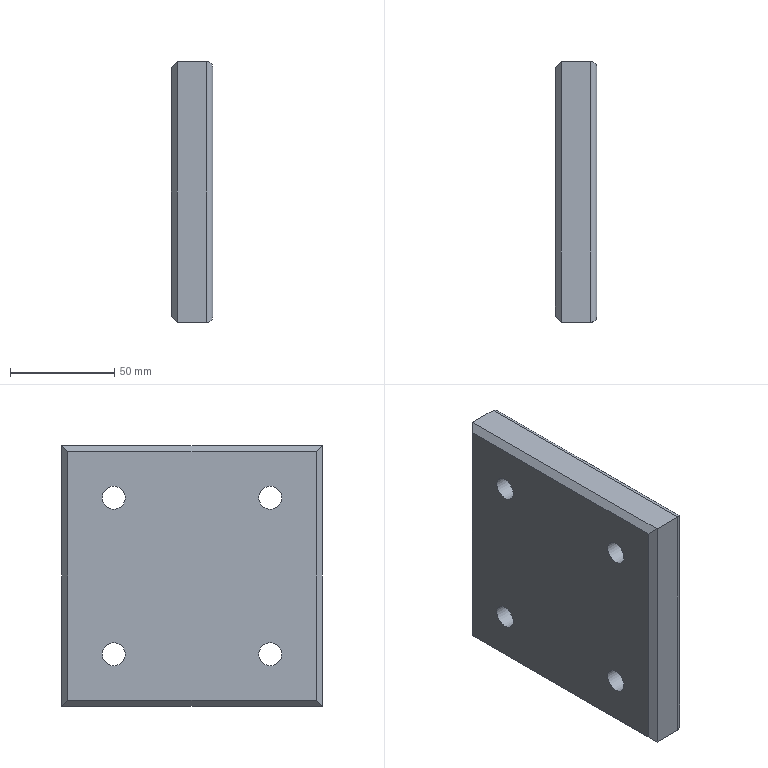Part | NX | features solid 2 | 1 solid | 26 faces | box 20 x 125 x 125 mm | volume 294744 mm3 | plane 14 | cylinder 12 | commonest cylinder face diameters 6 x4 11 x4 17.5 x4
STEP:
#1=CARTESIAN_POINT('',(993.,-247.5,-240.));
#2=VERTEX_POINT('',#1);
#3=CARTESIAN_POINT('',(1007.,-247.5,-240.));
#4=VERTEX_POINT('',#3);
#5=CARTESIAN_POINT('',(990.,-247.5,-240.));
#6=DIRECTION('',(1.,0.,0.));
#7=VECTOR('',#6,1000.);
#8=LINE('',#5,#7);
#9=EDGE_CURVE('',#2,#4,#8,.T.);
#10=ORIENTED_EDGE('',*,*,#9,.T.);
#11=CARTESIAN_POINT('',(1007.,-372.5,-240.));
#12=VERTEX_POINT('',#11);
#13=CARTESIAN_POINT('',(1007.,-272.5,-240.));
#14=DIRECTION('',(0.,1.,0.));
#15=VECTOR('',#14,1000.);
#16=LINE('',#13,#15);
#17=EDGE_CURVE('',#12,#4,#16,.T.);
#18=ORIENTED_EDGE('',*,*,#17,.F.);
#19=CARTESIAN_POINT('',(993.,-372.5,-240.));
#20=VERTEX_POINT('',#19);
#21=CARTESIAN_POINT('',(990.,-372.5,-240.));
#22=DIRECTION('',(1.,0.,0.));
#23=VECTOR('',#22,1000.);
#24=LINE('',#21,#23);
#25=EDGE_CURVE('',#20,#12,#24,.T.);
#26=ORIENTED_EDGE('',*,*,#25,.F.);
#27=CARTESIAN_POINT('',(993.,-372.5,-240.));
#28=DIRECTION('',(0.,-1.,0.));
#29=VECTOR('',#28,1000.);
#30=LINE('',#27,#29);
#31=EDGE_CURVE('',#2,#20,#30,.T.);
#32=ORIENTED_EDGE('',*,*,#31,.F.);
#33=EDGE_LOOP('',(#10,#18,#26,#32));
#34=FACE_BOUND('',#33,.T.);
#35=CARTESIAN_POINT('',(990.,-372.5,-240.));
#36=DIRECTION('',(0.,0.,1.));
#37=DIRECTION('',(0.,-1.,0.));
#38=AXIS2_PLACEMENT_3D('',#35,#36,#37);
#39=PLANE('',#38);
#40=ADVANCED_FACE('',(#34),#39,.F.);
#41=CARTESIAN_POINT('',(993.,-247.5,-115.));
#42=VERTEX_POINT('',#41);
#43=CARTESIAN_POINT('',(1007.,-247.5,-115.));
#44=VERTEX_POINT('',#43);
#45=CARTESIAN_POINT('',(990.,-247.5,-115.));
#46=DIRECTION('',(1.,0.,0.));
#47=VECTOR('',#46,1000.);
#48=LINE('',#45,#47);
#49=EDGE_CURVE('',#42,#44,#48,.T.);
#50=ORIENTED_EDGE('',*,*,#49,.T.);
#51=CARTESIAN_POINT('',(1007.,-247.5,-115.));
#52=DIRECTION('',(0.,0.,1.));
#53=VECTOR('',#52,1000.);
#54=LINE('',#51,#53);
#55=EDGE_CURVE('',#4,#44,#54,.T.);
#56=ORIENTED_EDGE('',*,*,#55,.F.);
#57=ORIENTED_EDGE('',*,*,#9,.F.);
#58=CARTESIAN_POINT('',(993.,-247.5,-240.));
#59=DIRECTION('',(0.,0.,-1.));
#60=VECTOR('',#59,1000.);
#61=LINE('',#58,#60);
#62=EDGE_CURVE('',#42,#2,#61,.T.);
#63=ORIENTED_EDGE('',*,*,#62,.F.);
#64=EDGE_LOOP('',(#50,#56,#57,#63));
#65=FACE_BOUND('',#64,.T.);
#66=CARTESIAN_POINT('',(990.,-247.5,-240.));
#67=DIRECTION('',(0.,-1.,0.));
#68=DIRECTION('',(0.,0.,-1.));
#69=AXIS2_PLACEMENT_3D('',#66,#67,#68);
#70=PLANE('',#69);
#71=ADVANCED_FACE('',(#65),#70,.F.);
#72=CARTESIAN_POINT('',(993.,-372.5,-115.));
#73=VERTEX_POINT('',#72);
#74=CARTESIAN_POINT('',(1007.,-372.5,-115.));
#75=VERTEX_POINT('',#74);
#76=CARTESIAN_POINT('',(990.,-372.5,-115.));
#77=DIRECTION('',(1.,0.,0.));
#78=VECTOR('',#77,1000.);
#79=LINE('',#76,#78);
#80=EDGE_CURVE('',#73,#75,#79,.T.);
#81=ORIENTED_EDGE('',*,*,#80,.T.);
#82=CARTESIAN_POINT('',(1007.,-372.5,-115.));
#83=DIRECTION('',(0.,-1.,0.));
#84=VECTOR('',#83,1000.);
#85=LINE('',#82,#84);
#86=EDGE_CURVE('',#44,#75,#85,.T.);
#87=ORIENTED_EDGE('',*,*,#86,.F.);
#88=ORIENTED_EDGE('',*,*,#49,.F.);
#89=CARTESIAN_POINT('',(993.,-272.5,-115.));
#90=DIRECTION('',(0.,1.,0.));
#91=VECTOR('',#90,1000.);
#92=LINE('',#89,#91);
#93=EDGE_CURVE('',#73,#42,#92,.T.);
#94=ORIENTED_EDGE('',*,*,#93,.F.);
#95=EDGE_LOOP('',(#81,#87,#88,#94));
#96=FACE_BOUND('',#95,.T.);
#97=CARTESIAN_POINT('',(990.,-272.5,-115.));
#98=DIRECTION('',(0.,0.,-1.));
#99=DIRECTION('',(-1.,0.,0.));
#100=AXIS2_PLACEMENT_3D('',#97,#98,#99);
#101=PLANE('',#100);
#102=ADVANCED_FACE('',(#96),#101,.F.);
#103=ORIENTED_EDGE('',*,*,#25,.T.);
#104=CARTESIAN_POINT('',(1007.,-372.5,-240.));
#105=DIRECTION('',(0.,0.,-1.));
#106=VECTOR('',#105,1000.);
#107=LINE('',#104,#106);
#108=EDGE_CURVE('',#75,#12,#107,.T.);
#109=ORIENTED_EDGE('',*,*,#108,.F.);
#110=ORIENTED_EDGE('',*,*,#80,.F.);
#111=CARTESIAN_POINT('',(993.,-372.5,-115.));
#112=DIRECTION('',(0.,0.,1.));
#113=VECTOR('',#112,1000.);
#114=LINE('',#111,#113);
#115=EDGE_CURVE('',#20,#73,#114,.T.);
#116=ORIENTED_EDGE('',*,*,#115,.F.);
#117=EDGE_LOOP('',(#103,#109,#110,#116));
#118=FACE_BOUND('',#117,.T.);
#119=CARTESIAN_POINT('',(990.,-372.5,-115.));
#120=DIRECTION('',(0.,1.,0.));
#121=DIRECTION('',(0.,0.,1.));
#122=AXIS2_PLACEMENT_3D('',#119,#120,#121);
#123=PLANE('',#122);
#124=ADVANCED_FACE('',(#118),#123,.F.);
#125=CARTESIAN_POINT('',(990.,-250.5,-237.));
#126=VERTEX_POINT('',#125);
#127=CARTESIAN_POINT('',(990.,-250.5,-118.));
#128=VERTEX_POINT('',#127);
#129=CARTESIAN_POINT('',(990.,-250.5,-240.));
#130=DIRECTION('',(0.,0.,1.));
#131=VECTOR('',#130,1000.);
#132=LINE('',#129,#131);
#133=EDGE_CURVE('',#126,#128,#132,.T.);
#134=ORIENTED_EDGE('',*,*,#133,.F.);
#135=CARTESIAN_POINT('',(990.,-369.5,-237.));
#136=VERTEX_POINT('',#135);
#137=CARTESIAN_POINT('',(990.,-372.5,-237.));
#138=DIRECTION('',(0.,1.,0.));
#139=VECTOR('',#138,1000.);
#140=LINE('',#137,#139);
#141=EDGE_CURVE('',#136,#126,#140,.T.);
#142=ORIENTED_EDGE('',*,*,#141,.F.);
#143=CARTESIAN_POINT('',(990.,-369.5,-118.));
#144=VERTEX_POINT('',#143);
#145=CARTESIAN_POINT('',(990.,-369.5,-240.));
#146=DIRECTION('',(0.,0.,-1.));
#147=VECTOR('',#146,1000.);
#148=LINE('',#145,#147);
#149=EDGE_CURVE('',#144,#136,#148,.T.);
#150=ORIENTED_EDGE('',*,*,#149,.F.);
#151=CARTESIAN_POINT('',(990.,-372.5,-118.));
#152=DIRECTION('',(0.,-1.,0.));
#153=VECTOR('',#152,1000.);
#154=LINE('',#151,#153);
#155=EDGE_CURVE('',#128,#144,#154,.T.);
#156=ORIENTED_EDGE('',*,*,#155,.F.);
#157=EDGE_LOOP('',(#134,#142,#150,#156));
#158=FACE_BOUND('',#157,.T.);
#159=CARTESIAN_POINT('',(990.,-272.5,-145.5));
#160=VERTEX_POINT('',#159);
#161=CARTESIAN_POINT('',(990.,-272.5,-140.));
#162=DIRECTION('',(-1.,0.,0.));
#163=DIRECTION('',(0.,0.,-1.));
#164=AXIS2_PLACEMENT_3D('',#161,#162,#163);
#165=CIRCLE('',#164,5.5);
#166=EDGE_CURVE('',#160,#160,#165,.T.);
#167=ORIENTED_EDGE('',*,*,#166,.F.);
#168=EDGE_LOOP('',(#167));
#169=FACE_BOUND('',#168,.T.);
#170=CARTESIAN_POINT('',(990.,-347.5,-145.5));
#171=VERTEX_POINT('',#170);
#172=CARTESIAN_POINT('',(990.,-347.5,-140.));
#173=DIRECTION('',(-1.,0.,0.));
#174=DIRECTION('',(0.,0.,-1.));
#175=AXIS2_PLACEMENT_3D('',#172,#173,#174);
#176=CIRCLE('',#175,5.5);
#177=EDGE_CURVE('',#171,#171,#176,.T.);
#178=ORIENTED_EDGE('',*,*,#177,.F.);
#179=EDGE_LOOP('',(#178));
#180=FACE_BOUND('',#179,.T.);
#181=CARTESIAN_POINT('',(990.,-272.5,-220.5));
#182=VERTEX_POINT('',#181);
#183=CARTESIAN_POINT('',(990.,-272.5,-215.));
#184=DIRECTION('',(-1.,0.,0.));
#185=DIRECTION('',(0.,0.,-1.));
#186=AXIS2_PLACEMENT_3D('',#183,#184,#185);
#187=CIRCLE('',#186,5.5);
#188=EDGE_CURVE('',#182,#182,#187,.T.);
#189=ORIENTED_EDGE('',*,*,#188,.F.);
#190=EDGE_LOOP('',(#189));
#191=FACE_BOUND('',#190,.T.);
#192=CARTESIAN_POINT('',(990.,-347.5,-220.5));
#193=VERTEX_POINT('',#192);
#194=CARTESIAN_POINT('',(990.,-347.5,-215.));
#195=DIRECTION('',(-1.,0.,0.));
#196=DIRECTION('',(0.,0.,-1.));
#197=AXIS2_PLACEMENT_3D('',#194,#195,#196);
#198=CIRCLE('',#197,5.5);
#199=EDGE_CURVE('',#193,#193,#198,.T.);
#200=ORIENTED_EDGE('',*,*,#199,.F.);
#201=EDGE_LOOP('',(#200));
#202=FACE_BOUND('',#201,.T.);
#203=CARTESIAN_POINT('',(990.,-372.5,-240.));
#204=DIRECTION('',(1.,0.,0.));
#205=DIRECTION('',(0.,0.,-1.));
#206=AXIS2_PLACEMENT_3D('',#203,#204,#205);
#207=PLANE('',#206);
#208=ADVANCED_FACE('',(#158,#169,#180,#191,#202),#207,.F.);
#209=CARTESIAN_POINT('',(1010.,-250.5,-237.));
#210=VERTEX_POINT('',#209);
#211=CARTESIAN_POINT('',(1010.,-369.5,-237.));
#212=VERTEX_POINT('',#211);
#213=CARTESIAN_POINT('',(1010.,-372.5,-237.));
#214=DIRECTION('',(0.,1.,0.));
#215=VECTOR('',#214,1000.);
#216=LINE('',#213,#215);
#217=EDGE_CURVE('',#210,#212,#216,.F.);
#218=ORIENTED_EDGE('',*,*,#217,.F.);
#219=CARTESIAN_POINT('',(1010.,-250.5,-118.));
#220=VERTEX_POINT('',#219);
#221=CARTESIAN_POINT('',(1010.,-250.5,-240.));
#222=DIRECTION('',(0.,0.,1.));
#223=VECTOR('',#222,1000.);
#224=LINE('',#221,#223);
#225=EDGE_CURVE('',#220,#210,#224,.F.);
#226=ORIENTED_EDGE('',*,*,#225,.F.);
#227=CARTESIAN_POINT('',(1010.,-369.5,-118.));
#228=VERTEX_POINT('',#227);
#229=CARTESIAN_POINT('',(1010.,-272.5,-118.));
#230=DIRECTION('',(0.,-1.,0.));
#231=VECTOR('',#230,1000.);
#232=LINE('',#229,#231);
#233=EDGE_CURVE('',#228,#220,#232,.F.);
#234=ORIENTED_EDGE('',*,*,#233,.F.);
#235=CARTESIAN_POINT('',(1010.,-369.5,-115.));
#236=DIRECTION('',(0.,0.,-1.));
#237=VECTOR('',#236,1000.);
#238=LINE('',#235,#237);
#239=EDGE_CURVE('',#212,#228,#238,.F.);
#240=ORIENTED_EDGE('',*,*,#239,.F.);
#241=EDGE_LOOP('',(#218,#226,#234,#240));
#242=FACE_BOUND('',#241,.T.);
#243=CARTESIAN_POINT('',(1010.,-272.5,-131.25));
#244=VERTEX_POINT('',#243);
#245=CARTESIAN_POINT('',(1010.,-272.5,-140.));
#246=DIRECTION('',(1.,0.,0.));
#247=DIRECTION('',(0.,0.,1.));
#248=AXIS2_PLACEMENT_3D('',#245,#246,#247);
#249=CIRCLE('',#248,8.75);
#250=EDGE_CURVE('',#244,#244,#249,.T.);
#251=ORIENTED_EDGE('',*,*,#250,.F.);
#252=EDGE_LOOP('',(#251));
#253=FACE_BOUND('',#252,.T.);
#254=CARTESIAN_POINT('',(1010.,-347.5,-131.25));
#255=VERTEX_POINT('',#254);
#256=CARTESIAN_POINT('',(1010.,-347.5,-140.));
#257=DIRECTION('',(1.,0.,0.));
#258=DIRECTION('',(0.,0.,1.));
#259=AXIS2_PLACEMENT_3D('',#256,#257,#258);
#260=CIRCLE('',#259,8.75);
#261=EDGE_CURVE('',#255,#255,#260,.T.);
#262=ORIENTED_EDGE('',*,*,#261,.F.);
#263=EDGE_LOOP('',(#262));
#264=FACE_BOUND('',#263,.T.);
#265=CARTESIAN_POINT('',(1010.,-272.5,-206.25));
#266=VERTEX_POINT('',#265);
#267=CARTESIAN_POINT('',(1010.,-272.5,-215.));
#268=DIRECTION('',(1.,0.,0.));
#269=DIRECTION('',(0.,0.,1.));
#270=AXIS2_PLACEMENT_3D('',#267,#268,#269);
#271=CIRCLE('',#270,8.75);
#272=EDGE_CURVE('',#266,#266,#271,.T.);
#273=ORIENTED_EDGE('',*,*,#272,.F.);
#274=EDGE_LOOP('',(#273));
#275=FACE_BOUND('',#274,.T.);
#276=CARTESIAN_POINT('',(1010.,-347.5,-206.25));
#277=VERTEX_POINT('',#276);
#278=CARTESIAN_POINT('',(1010.,-347.5,-215.));
#279=DIRECTION('',(1.,0.,0.));
#280=DIRECTION('',(0.,0.,1.));
#281=AXIS2_PLACEMENT_3D('',#278,#279,#280);
#282=CIRCLE('',#281,8.75);
#283=EDGE_CURVE('',#277,#277,#282,.T.);
#284=ORIENTED_EDGE('',*,*,#283,.F.);
#285=EDGE_LOOP('',(#284));
#286=FACE_BOUND('',#285,.T.);
#287=CARTESIAN_POINT('',(1010.,-372.5,-240.));
#288=DIRECTION('',(1.,0.,0.));
#289=DIRECTION('',(0.,0.,-1.));
#290=AXIS2_PLACEMENT_3D('',#287,#288,#289);
#291=PLANE('',#290);
#292=ADVANCED_FACE('',(#242,#253,#264,#275,#286),#291,.T.);
#293=CARTESIAN_POINT('',(998.,-347.5,-209.5));
#294=VERTEX_POINT('',#293);
#295=CARTESIAN_POINT('',(998.,-347.5,-215.));
#296=DIRECTION('',(1.,0.,0.));
#297=DIRECTION('',(0.,0.,1.));
#298=AXIS2_PLACEMENT_3D('',#295,#296,#297);
#299=CIRCLE('',#298,5.5);
#300=EDGE_CURVE('',#294,#294,#299,.T.);
#301=ORIENTED_EDGE('',*,*,#300,.T.);
#302=EDGE_LOOP('',(#301));
#303=FACE_BOUND('',#302,.T.);
#304=ORIENTED_EDGE('',*,*,#199,.T.);
#305=EDGE_LOOP('',(#304));
#306=FACE_BOUND('',#305,.T.);
#307=CARTESIAN_POINT('',(960.,-347.5,-215.));
#308=DIRECTION('',(-1.,0.,0.));
#309=DIRECTION('',(0.,0.,1.));
#310=AXIS2_PLACEMENT_3D('',#307,#308,#309);
#311=CYLINDRICAL_SURFACE('',#310,5.5);
#312=ADVANCED_FACE('',(#303,#306),#311,.F.);
#313=ORIENTED_EDGE('',*,*,#300,.F.);
#314=EDGE_LOOP('',(#313));
#315=FACE_BOUND('',#314,.T.);
#316=CARTESIAN_POINT('',(998.,-347.5,-206.25));
#317=VERTEX_POINT('',#316);
#318=CARTESIAN_POINT('',(998.,-347.5,-215.));
#319=DIRECTION('',(1.,0.,0.));
#320=DIRECTION('',(0.,0.,1.));
#321=AXIS2_PLACEMENT_3D('',#318,#319,#320);
#322=CIRCLE('',#321,8.75);
#323=EDGE_CURVE('',#317,#317,#322,.T.);
#324=ORIENTED_EDGE('',*,*,#323,.T.);
#325=EDGE_LOOP('',(#324));
#326=FACE_BOUND('',#325,.T.);
#327=CARTESIAN_POINT('',(998.,-347.5,-215.));
#328=DIRECTION('',(-1.,0.,0.));
#329=DIRECTION('',(0.,0.,1.));
#330=AXIS2_PLACEMENT_3D('',#327,#328,#329);
#331=PLANE('',#330);
#332=ADVANCED_FACE('',(#315,#326),#331,.F.);
#333=ORIENTED_EDGE('',*,*,#323,.F.);
#334=EDGE_LOOP('',(#333));
#335=FACE_BOUND('',#334,.T.);
#336=ORIENTED_EDGE('',*,*,#283,.T.);
#337=EDGE_LOOP('',(#336));
#338=FACE_BOUND('',#337,.T.);
#339=CARTESIAN_POINT('',(1010.,-347.5,-215.));
#340=DIRECTION('',(-1.,0.,0.));
#341=DIRECTION('',(0.,0.,1.));
#342=AXIS2_PLACEMENT_3D('',#339,#340,#341);
#343=CYLINDRICAL_SURFACE('',#342,8.75);
#344=ADVANCED_FACE('',(#335,#338),#343,.F.);
#345=CARTESIAN_POINT('',(998.,-272.5,-209.5));
#346=VERTEX_POINT('',#345);
#347=CARTESIAN_POINT('',(998.,-272.5,-215.));
#348=DIRECTION('',(1.,0.,0.));
#349=DIRECTION('',(0.,0.,1.));
#350=AXIS2_PLACEMENT_3D('',#347,#348,#349);
#351=CIRCLE('',#350,5.5);
#352=EDGE_CURVE('',#346,#346,#351,.T.);
#353=ORIENTED_EDGE('',*,*,#352,.T.);
#354=EDGE_LOOP('',(#353));
#355=FACE_BOUND('',#354,.T.);
#356=ORIENTED_EDGE('',*,*,#188,.T.);
#357=EDGE_LOOP('',(#356));
#358=FACE_BOUND('',#357,.T.);
#359=CARTESIAN_POINT('',(960.,-272.5,-215.));
#360=DIRECTION('',(-1.,0.,0.));
#361=DIRECTION('',(0.,0.,1.));
#362=AXIS2_PLACEMENT_3D('',#359,#360,#361);
#363=CYLINDRICAL_SURFACE('',#362,5.5);
#364=ADVANCED_FACE('',(#355,#358),#363,.F.);
#365=ORIENTED_EDGE('',*,*,#352,.F.);
#366=EDGE_LOOP('',(#365));
#367=FACE_BOUND('',#366,.T.);
#368=CARTESIAN_POINT('',(998.,-272.5,-206.25));
#369=VERTEX_POINT('',#368);
#370=CARTESIAN_POINT('',(998.,-272.5,-215.));
#371=DIRECTION('',(1.,0.,0.));
#372=DIRECTION('',(0.,0.,1.));
#373=AXIS2_PLACEMENT_3D('',#370,#371,#372);
#374=CIRCLE('',#373,8.75);
#375=EDGE_CURVE('',#369,#369,#374,.T.);
#376=ORIENTED_EDGE('',*,*,#375,.T.);
#377=EDGE_LOOP('',(#376));
#378=FACE_BOUND('',#377,.T.);
#379=CARTESIAN_POINT('',(998.,-272.5,-215.));
#380=DIRECTION('',(-1.,0.,0.));
#381=DIRECTION('',(0.,0.,1.));
#382=AXIS2_PLACEMENT_3D('',#379,#380,#381);
#383=PLANE('',#382);
#384=ADVANCED_FACE('',(#367,#378),#383,.F.);
#385=ORIENTED_EDGE('',*,*,#375,.F.);
#386=EDGE_LOOP('',(#385));
#387=FACE_BOUND('',#386,.T.);
#388=ORIENTED_EDGE('',*,*,#272,.T.);
#389=EDGE_LOOP('',(#388));
#390=FACE_BOUND('',#389,.T.);
#391=CARTESIAN_POINT('',(1010.,-272.5,-215.));
#392=DIRECTION('',(-1.,0.,0.));
#393=DIRECTION('',(0.,0.,1.));
#394=AXIS2_PLACEMENT_3D('',#391,#392,#393);
#395=CYLINDRICAL_SURFACE('',#394,8.75);
#396=ADVANCED_FACE('',(#387,#390),#395,.F.);
#397=CARTESIAN_POINT('',(998.,-347.5,-134.5));
#398=VERTEX_POINT('',#397);
#399=CARTESIAN_POINT('',(998.,-347.5,-140.));
#400=DIRECTION('',(1.,0.,0.));
#401=DIRECTION('',(0.,0.,1.));
#402=AXIS2_PLACEMENT_3D('',#399,#400,#401);
#403=CIRCLE('',#402,5.5);
#404=EDGE_CURVE('',#398,#398,#403,.T.);
#405=ORIENTED_EDGE('',*,*,#404,.T.);
#406=EDGE_LOOP('',(#405));
#407=FACE_BOUND('',#406,.T.);
#408=ORIENTED_EDGE('',*,*,#177,.T.);
#409=EDGE_LOOP('',(#408));
#410=FACE_BOUND('',#409,.T.);
#411=CARTESIAN_POINT('',(960.,-347.5,-140.));
#412=DIRECTION('',(-1.,0.,0.));
#413=DIRECTION('',(0.,0.,1.));
#414=AXIS2_PLACEMENT_3D('',#411,#412,#413);
#415=CYLINDRICAL_SURFACE('',#414,5.5);
#416=ADVANCED_FACE('',(#407,#410),#415,.F.);
#417=ORIENTED_EDGE('',*,*,#404,.F.);
#418=EDGE_LOOP('',(#417));
#419=FACE_BOUND('',#418,.T.);
#420=CARTESIAN_POINT('',(998.,-347.5,-131.25));
#421=VERTEX_POINT('',#420);
#422=CARTESIAN_POINT('',(998.,-347.5,-140.));
#423=DIRECTION('',(1.,0.,0.));
#424=DIRECTION('',(0.,0.,1.));
#425=AXIS2_PLACEMENT_3D('',#422,#423,#424);
#426=CIRCLE('',#425,8.75);
#427=EDGE_CURVE('',#421,#421,#426,.T.);
#428=ORIENTED_EDGE('',*,*,#427,.T.);
#429=EDGE_LOOP('',(#428));
#430=FACE_BOUND('',#429,.T.);
#431=CARTESIAN_POINT('',(998.,-347.5,-140.));
#432=DIRECTION('',(-1.,0.,0.));
#433=DIRECTION('',(0.,0.,1.));
#434=AXIS2_PLACEMENT_3D('',#431,#432,#433);
#435=PLANE('',#434);
#436=ADVANCED_FACE('',(#419,#430),#435,.F.);
#437=ORIENTED_EDGE('',*,*,#427,.F.);
#438=EDGE_LOOP('',(#437));
#439=FACE_BOUND('',#438,.T.);
#440=ORIENTED_EDGE('',*,*,#261,.T.);
#441=EDGE_LOOP('',(#440));
#442=FACE_BOUND('',#441,.T.);
#443=CARTESIAN_POINT('',(1010.,-347.5,-140.));
#444=DIRECTION('',(-1.,0.,0.));
#445=DIRECTION('',(0.,0.,1.));
#446=AXIS2_PLACEMENT_3D('',#443,#444,#445);
#447=CYLINDRICAL_SURFACE('',#446,8.75);
#448=ADVANCED_FACE('',(#439,#442),#447,.F.);
#449=CARTESIAN_POINT('',(998.,-272.5,-134.5));
#450=VERTEX_POINT('',#449);
#451=CARTESIAN_POINT('',(998.,-272.5,-140.));
#452=DIRECTION('',(1.,0.,0.));
#453=DIRECTION('',(0.,0.,1.));
#454=AXIS2_PLACEMENT_3D('',#451,#452,#453);
#455=CIRCLE('',#454,5.5);
#456=EDGE_CURVE('',#450,#450,#455,.T.);
#457=ORIENTED_EDGE('',*,*,#456,.T.);
#458=EDGE_LOOP('',(#457));
#459=FACE_BOUND('',#458,.T.);
#460=ORIENTED_EDGE('',*,*,#166,.T.);
#461=EDGE_LOOP('',(#460));
#462=FACE_BOUND('',#461,.T.);
#463=CARTESIAN_POINT('',(960.,-272.5,-140.));
#464=DIRECTION('',(-1.,0.,0.));
#465=DIRECTION('',(0.,0.,1.));
#466=AXIS2_PLACEMENT_3D('',#463,#464,#465);
#467=CYLINDRICAL_SURFACE('',#466,5.5);
#468=ADVANCED_FACE('',(#459,#462),#467,.F.);
#469=ORIENTED_EDGE('',*,*,#456,.F.);
#470=EDGE_LOOP('',(#469));
#471=FACE_BOUND('',#470,.T.);
#472=CARTESIAN_POINT('',(998.,-272.5,-131.25));
#473=VERTEX_POINT('',#472);
#474=CARTESIAN_POINT('',(998.,-272.5,-140.));
#475=DIRECTION('',(1.,0.,0.));
#476=DIRECTION('',(0.,0.,1.));
#477=AXIS2_PLACEMENT_3D('',#474,#475,#476);
#478=CIRCLE('',#477,8.75);
#479=EDGE_CURVE('',#473,#473,#478,.T.);
#480=ORIENTED_EDGE('',*,*,#479,.T.);
#481=EDGE_LOOP('',(#480));
#482=FACE_BOUND('',#481,.T.);
#483=CARTESIAN_POINT('',(998.,-272.5,-140.));
#484=DIRECTION('',(-1.,0.,0.));
#485=DIRECTION('',(0.,0.,1.));
#486=AXIS2_PLACEMENT_3D('',#483,#484,#485);
#487=PLANE('',#486);
#488=ADVANCED_FACE('',(#471,#482),#487,.F.);
#489=ORIENTED_EDGE('',*,*,#479,.F.);
#490=EDGE_LOOP('',(#489));
#491=FACE_BOUND('',#490,.T.);
#492=ORIENTED_EDGE('',*,*,#250,.T.);
#493=EDGE_LOOP('',(#492));
#494=FACE_BOUND('',#493,.T.);
#495=CARTESIAN_POINT('',(1010.,-272.5,-140.));
#496=DIRECTION('',(-1.,0.,0.));
#497=DIRECTION('',(0.,0.,1.));
#498=AXIS2_PLACEMENT_3D('',#495,#496,#497);
#499=CYLINDRICAL_SURFACE('',#498,8.75);
#500=ADVANCED_FACE('',(#491,#494),#499,.F.);
#501=CARTESIAN_POINT('',(1007.,-250.5,-237.));
#502=DIRECTION('',(0.,0.7071,0.7071));
#503=DIRECTION('',(0.,-0.7071,0.7071));
#504=AXIS2_PLACEMENT_3D('',#501,#502,#503);
#505=ELLIPSE('',#504,4.243,3.);
#506=EDGE_CURVE('',#210,#4,#505,.T.);
#507=ORIENTED_EDGE('',*,*,#506,.T.);
#508=ORIENTED_EDGE('',*,*,#55,.T.);
#509=CARTESIAN_POINT('',(1007.,-250.5,-118.));
#510=DIRECTION('',(0.,-0.7071,0.7071));
#511=DIRECTION('',(0.,-0.7071,-0.7071));
#512=AXIS2_PLACEMENT_3D('',#509,#510,#511);
#513=ELLIPSE('',#512,4.243,3.);
#514=EDGE_CURVE('',#44,#220,#513,.F.);
#515=ORIENTED_EDGE('',*,*,#514,.T.);
#516=ORIENTED_EDGE('',*,*,#225,.T.);
#517=EDGE_LOOP('',(#507,#508,#515,#516));
#518=FACE_BOUND('',#517,.T.);
#519=CARTESIAN_POINT('',(1007.,-250.5,-240.));
#520=DIRECTION('',(0.,0.,-1.));
#521=DIRECTION('',(0.,1.,0.));
#522=AXIS2_PLACEMENT_3D('',#519,#520,#521);
#523=CYLINDRICAL_SURFACE('',#522,3.);
#524=ADVANCED_FACE('',(#518),#523,.T.);
#525=ORIENTED_EDGE('',*,*,#514,.F.);
#526=ORIENTED_EDGE('',*,*,#86,.T.);
#527=CARTESIAN_POINT('',(1007.,-369.5,-118.));
#528=DIRECTION('',(0.,-0.7071,-0.7071));
#529=DIRECTION('',(0.,0.7071,-0.7071));
#530=AXIS2_PLACEMENT_3D('',#527,#528,#529);
#531=ELLIPSE('',#530,4.243,3.);
#532=EDGE_CURVE('',#75,#228,#531,.F.);
#533=ORIENTED_EDGE('',*,*,#532,.T.);
#534=ORIENTED_EDGE('',*,*,#233,.T.);
#535=EDGE_LOOP('',(#525,#526,#533,#534));
#536=FACE_BOUND('',#535,.T.);
#537=CARTESIAN_POINT('',(1007.,-272.5,-118.));
#538=DIRECTION('',(0.,1.,0.));
#539=DIRECTION('',(1.,0.,0.));
#540=AXIS2_PLACEMENT_3D('',#537,#538,#539);
#541=CYLINDRICAL_SURFACE('',#540,3.);
#542=ADVANCED_FACE('',(#536),#541,.T.);
#543=ORIENTED_EDGE('',*,*,#506,.F.);
#544=ORIENTED_EDGE('',*,*,#217,.T.);
#545=CARTESIAN_POINT('',(1007.,-369.5,-237.));
#546=DIRECTION('',(0.,0.7071,-0.7071));
#547=DIRECTION('',(0.,-0.7071,-0.7071));
#548=AXIS2_PLACEMENT_3D('',#545,#546,#547);
#549=ELLIPSE('',#548,4.243,3.);
#550=EDGE_CURVE('',#212,#12,#549,.T.);
#551=ORIENTED_EDGE('',*,*,#550,.T.);
#552=ORIENTED_EDGE('',*,*,#17,.T.);
#553=EDGE_LOOP('',(#543,#544,#551,#552));
#554=FACE_BOUND('',#553,.T.);
#555=CARTESIAN_POINT('',(1007.,-372.5,-237.));
#556=DIRECTION('',(0.,-1.,0.));
#557=DIRECTION('',(0.,0.,-1.));
#558=AXIS2_PLACEMENT_3D('',#555,#556,#557);
#559=CYLINDRICAL_SURFACE('',#558,3.);
#560=ADVANCED_FACE('',(#554),#559,.T.);
#561=ORIENTED_EDGE('',*,*,#532,.F.);
#562=ORIENTED_EDGE('',*,*,#108,.T.);
#563=ORIENTED_EDGE('',*,*,#550,.F.);
#564=ORIENTED_EDGE('',*,*,#239,.T.);
#565=EDGE_LOOP('',(#561,#562,#563,#564));
#566=FACE_BOUND('',#565,.T.);
#567=CARTESIAN_POINT('',(1007.,-369.5,-115.));
#568=DIRECTION('',(0.,0.,1.));
#569=DIRECTION('',(0.,-1.,0.));
#570=AXIS2_PLACEMENT_3D('',#567,#568,#569);
#571=CYLINDRICAL_SURFACE('',#570,3.);
#572=ADVANCED_FACE('',(#566),#571,.T.);
#573=CARTESIAN_POINT('',(991.,-370.5,-238.));
#574=DIRECTION('',(-0.5774,0.5774,0.5774));
#575=VECTOR('',#574,1000.);
#576=LINE('',#573,#575);
#577=EDGE_CURVE('',#20,#136,#576,.T.);
#578=ORIENTED_EDGE('',*,*,#577,.T.);
#579=ORIENTED_EDGE('',*,*,#141,.T.);
#580=CARTESIAN_POINT('',(957.667,-282.833,-204.667));
#581=DIRECTION('',(-0.5774,-0.5774,0.5774));
#582=VECTOR('',#581,1000.);
#583=LINE('',#580,#582);
#584=EDGE_CURVE('',#126,#2,#583,.F.);
#585=ORIENTED_EDGE('',*,*,#584,.T.);
#586=ORIENTED_EDGE('',*,*,#31,.T.);
#587=EDGE_LOOP('',(#578,#579,#585,#586));
#588=FACE_BOUND('',#587,.T.);
#589=CARTESIAN_POINT('',(990.,-372.5,-237.));
#590=DIRECTION('',(0.7071,0.,0.7071));
#591=DIRECTION('',(0.7071,0.,-0.7071));
#592=AXIS2_PLACEMENT_3D('',#589,#590,#591);
#593=PLANE('',#592);
#594=ADVANCED_FACE('',(#588),#593,.F.);
#595=ORIENTED_EDGE('',*,*,#584,.F.);
#596=ORIENTED_EDGE('',*,*,#133,.T.);
#597=CARTESIAN_POINT('',(949.333,-291.167,-158.667));
#598=DIRECTION('',(-0.5774,-0.5774,-0.5774));
#599=VECTOR('',#598,1000.);
#600=LINE('',#597,#599);
#601=EDGE_CURVE('',#128,#42,#600,.F.);
#602=ORIENTED_EDGE('',*,*,#601,.T.);
#603=ORIENTED_EDGE('',*,*,#62,.T.);
#604=EDGE_LOOP('',(#595,#596,#602,#603));
#605=FACE_BOUND('',#604,.T.);
#606=CARTESIAN_POINT('',(990.,-250.5,-240.));
#607=DIRECTION('',(0.7071,-0.7071,0.));
#608=DIRECTION('',(-0.7071,-0.7071,0.));
#609=AXIS2_PLACEMENT_3D('',#606,#607,#608);
#610=PLANE('',#609);
#611=ADVANCED_FACE('',(#605),#610,.F.);
#612=ORIENTED_EDGE('',*,*,#577,.F.);
#613=ORIENTED_EDGE('',*,*,#115,.T.);
#614=CARTESIAN_POINT('',(949.333,-328.833,-158.667));
#615=DIRECTION('',(0.5774,-0.5774,0.5774));
#616=VECTOR('',#615,1000.);
#617=LINE('',#614,#616);
#618=EDGE_CURVE('',#73,#144,#617,.F.);
#619=ORIENTED_EDGE('',*,*,#618,.T.);
#620=ORIENTED_EDGE('',*,*,#149,.T.);
#621=EDGE_LOOP('',(#612,#613,#619,#620));
#622=FACE_BOUND('',#621,.T.);
#623=CARTESIAN_POINT('',(990.,-369.5,-240.));
#624=DIRECTION('',(0.7071,0.7071,0.));
#625=DIRECTION('',(0.7071,-0.7071,0.));
#626=AXIS2_PLACEMENT_3D('',#623,#624,#625);
#627=PLANE('',#626);
#628=ADVANCED_FACE('',(#622),#627,.F.);
#629=ORIENTED_EDGE('',*,*,#601,.F.);
#630=ORIENTED_EDGE('',*,*,#155,.T.);
#631=ORIENTED_EDGE('',*,*,#618,.F.);
#632=ORIENTED_EDGE('',*,*,#93,.T.);
#633=EDGE_LOOP('',(#629,#630,#631,#632));
#634=FACE_BOUND('',#633,.T.);
#635=CARTESIAN_POINT('',(990.,-372.5,-118.));
#636=DIRECTION('',(0.7071,0.,-0.7071));
#637=DIRECTION('',(-0.7071,0.,-0.7071));
#638=AXIS2_PLACEMENT_3D('',#635,#636,#637);
#639=PLANE('',#638);
#640=ADVANCED_FACE('',(#634),#639,.F.);
#641=CLOSED_SHELL('',(#40,#71,#102,#124,#208,#292,#312,#332,#344,#364,#384,#396,#416,#436,#448,#468,#488,#500,#524,#542,#560,#572,#594,#611,#628,#640));
#642=MANIFOLD_SOLID_BREP('',#641);
#643=(LENGTH_UNIT()NAMED_UNIT(*)SI_UNIT(.MILLI.,.METRE.));
#644=UNCERTAINTY_MEASURE_WITH_UNIT(LENGTH_MEASURE(0.00001),#643,'','');
#645=(NAMED_UNIT(*)PLANE_ANGLE_UNIT()SI_UNIT($,.RADIAN.));
#646=(NAMED_UNIT(*)SI_UNIT($,.STERADIAN.)SOLID_ANGLE_UNIT());
#647=(GEOMETRIC_REPRESENTATION_CONTEXT(3)GLOBAL_UNCERTAINTY_ASSIGNED_CONTEXT((#644))GLOBAL_UNIT_ASSIGNED_CONTEXT((#643,#645,#646))REPRESENTATION_CONTEXT('',''));
#648=ADVANCED_BREP_SHAPE_REPRESENTATION('',(#642),#647);